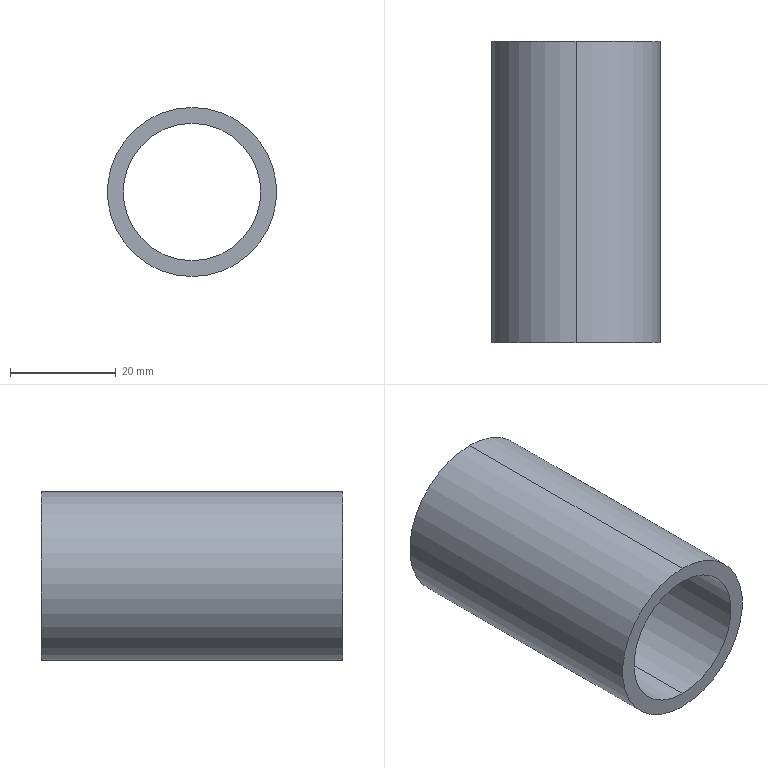Part | SolidWorks | features Chamfer 1, Extrusion 1 | 1 solid | 6 faces | box 32 x 57 x 32 mm | volume 15579 mm3 | cylinder 4 | plane 2 | commonest cylinder face diameters 26 x2 32 x2
STEP:
#1=CARTESIAN_POINT('',(0.,57.,-13.));
#2=VERTEX_POINT('',#1);
#3=CARTESIAN_POINT('',(0.,57.,13.));
#4=VERTEX_POINT('',#3);
#5=CARTESIAN_POINT('',(0.,57.,0.));
#6=DIRECTION('',(0.,1.,0.));
#7=DIRECTION('',(0.,0.,1.));
#8=AXIS2_PLACEMENT_3D('',#5,#6,#7);
#9=CIRCLE('',#8,13.);
#10=EDGE_CURVE('',#2,#4,#9,.T.);
#11=ORIENTED_EDGE('',*,*,#10,.T.);
#12=CARTESIAN_POINT('',(0.,0.,13.));
#13=VERTEX_POINT('',#12);
#14=CARTESIAN_POINT('',(0.,57.,13.));
#15=DIRECTION('',(0.,-1.,0.));
#16=VECTOR('',#15,1000.);
#17=LINE('',#14,#16);
#18=EDGE_CURVE('',#4,#13,#17,.T.);
#19=ORIENTED_EDGE('',*,*,#18,.T.);
#20=CARTESIAN_POINT('',(0.,0.,-13.));
#21=VERTEX_POINT('',#20);
#22=CARTESIAN_POINT('',(0.,0.,0.));
#23=DIRECTION('',(0.,1.,0.));
#24=DIRECTION('',(0.,0.,1.));
#25=AXIS2_PLACEMENT_3D('',#22,#23,#24);
#26=CIRCLE('',#25,13.);
#27=EDGE_CURVE('',#21,#13,#26,.T.);
#28=ORIENTED_EDGE('',*,*,#27,.F.);
#29=CARTESIAN_POINT('',(0.,57.,-13.));
#30=DIRECTION('',(0.,-1.,0.));
#31=VECTOR('',#30,1000.);
#32=LINE('',#29,#31);
#33=EDGE_CURVE('',#2,#21,#32,.T.);
#34=ORIENTED_EDGE('',*,*,#33,.F.);
#35=EDGE_LOOP('',(#11,#19,#28,#34));
#36=FACE_OUTER_BOUND('',#35,.T.);
#37=CARTESIAN_POINT('',(0.,57.,0.));
#38=DIRECTION('',(0.,-1.,0.));
#39=DIRECTION('',(0.,0.,-1.));
#40=AXIS2_PLACEMENT_3D('',#37,#38,#39);
#41=CYLINDRICAL_SURFACE('',#40,13.);
#42=ADVANCED_FACE('',(#36),#41,.F.);
#43=CARTESIAN_POINT('',(0.,57.,16.));
#44=VERTEX_POINT('',#43);
#45=CARTESIAN_POINT('',(0.,57.,-16.));
#46=VERTEX_POINT('',#45);
#47=CARTESIAN_POINT('',(0.,57.,0.));
#48=DIRECTION('',(0.,1.,0.));
#49=DIRECTION('',(0.,0.,1.));
#50=AXIS2_PLACEMENT_3D('',#47,#48,#49);
#51=CIRCLE('',#50,16.);
#52=EDGE_CURVE('',#44,#46,#51,.T.);
#53=ORIENTED_EDGE('',*,*,#52,.F.);
#54=CARTESIAN_POINT('',(0.,0.,16.));
#55=VERTEX_POINT('',#54);
#56=CARTESIAN_POINT('',(0.,57.,16.));
#57=DIRECTION('',(0.,-1.,0.));
#58=VECTOR('',#57,1000.);
#59=LINE('',#56,#58);
#60=EDGE_CURVE('',#44,#55,#59,.T.);
#61=ORIENTED_EDGE('',*,*,#60,.T.);
#62=CARTESIAN_POINT('',(0.,0.,-16.));
#63=VERTEX_POINT('',#62);
#64=CARTESIAN_POINT('',(0.,0.,0.));
#65=DIRECTION('',(0.,1.,0.));
#66=DIRECTION('',(0.,0.,1.));
#67=AXIS2_PLACEMENT_3D('',#64,#65,#66);
#68=CIRCLE('',#67,16.);
#69=EDGE_CURVE('',#55,#63,#68,.T.);
#70=ORIENTED_EDGE('',*,*,#69,.T.);
#71=CARTESIAN_POINT('',(0.,57.,-16.));
#72=DIRECTION('',(0.,-1.,0.));
#73=VECTOR('',#72,1000.);
#74=LINE('',#71,#73);
#75=EDGE_CURVE('',#46,#63,#74,.T.);
#76=ORIENTED_EDGE('',*,*,#75,.F.);
#77=EDGE_LOOP('',(#53,#61,#70,#76));
#78=FACE_OUTER_BOUND('',#77,.T.);
#79=CARTESIAN_POINT('',(0.,57.,0.));
#80=DIRECTION('',(0.,-1.,0.));
#81=DIRECTION('',(0.,0.,-1.));
#82=AXIS2_PLACEMENT_3D('',#79,#80,#81);
#83=CYLINDRICAL_SURFACE('',#82,16.);
#84=ADVANCED_FACE('',(#78),#83,.T.);
#85=CARTESIAN_POINT('',(0.,57.,0.));
#86=DIRECTION('',(0.,1.,0.));
#87=DIRECTION('',(0.,0.,1.));
#88=AXIS2_PLACEMENT_3D('',#85,#86,#87);
#89=CIRCLE('',#88,16.);
#90=EDGE_CURVE('',#46,#44,#89,.T.);
#91=ORIENTED_EDGE('',*,*,#90,.T.);
#92=ORIENTED_EDGE('',*,*,#52,.T.);
#93=EDGE_LOOP('',(#91,#92));
#94=FACE_OUTER_BOUND('',#93,.T.);
#95=ORIENTED_EDGE('',*,*,#10,.F.);
#96=CARTESIAN_POINT('',(0.,57.,0.));
#97=DIRECTION('',(0.,1.,0.));
#98=DIRECTION('',(0.,0.,1.));
#99=AXIS2_PLACEMENT_3D('',#96,#97,#98);
#100=CIRCLE('',#99,13.);
#101=EDGE_CURVE('',#4,#2,#100,.T.);
#102=ORIENTED_EDGE('',*,*,#101,.F.);
#103=EDGE_LOOP('',(#95,#102));
#104=FACE_BOUND('',#103,.T.);
#105=CARTESIAN_POINT('',(0.,57.,0.));
#106=DIRECTION('',(0.,1.,0.));
#107=DIRECTION('',(0.,0.,1.));
#108=AXIS2_PLACEMENT_3D('',#105,#106,#107);
#109=PLANE('',#108);
#110=ADVANCED_FACE('',(#94,#104),#109,.T.);
#111=CARTESIAN_POINT('',(0.,0.,0.));
#112=DIRECTION('',(0.,1.,0.));
#113=DIRECTION('',(0.,0.,1.));
#114=AXIS2_PLACEMENT_3D('',#111,#112,#113);
#115=CIRCLE('',#114,16.);
#116=EDGE_CURVE('',#63,#55,#115,.T.);
#117=ORIENTED_EDGE('',*,*,#116,.F.);
#118=ORIENTED_EDGE('',*,*,#69,.F.);
#119=EDGE_LOOP('',(#117,#118));
#120=FACE_OUTER_BOUND('',#119,.T.);
#121=ORIENTED_EDGE('',*,*,#27,.T.);
#122=CARTESIAN_POINT('',(0.,0.,0.));
#123=DIRECTION('',(0.,1.,0.));
#124=DIRECTION('',(0.,0.,1.));
#125=AXIS2_PLACEMENT_3D('',#122,#123,#124);
#126=CIRCLE('',#125,13.);
#127=EDGE_CURVE('',#13,#21,#126,.T.);
#128=ORIENTED_EDGE('',*,*,#127,.T.);
#129=EDGE_LOOP('',(#121,#128));
#130=FACE_BOUND('',#129,.T.);
#131=CARTESIAN_POINT('',(0.,0.,0.));
#132=DIRECTION('',(0.,1.,0.));
#133=DIRECTION('',(0.,0.,1.));
#134=AXIS2_PLACEMENT_3D('',#131,#132,#133);
#135=PLANE('',#134);
#136=ADVANCED_FACE('',(#120,#130),#135,.F.);
#137=ORIENTED_EDGE('',*,*,#60,.F.);
#138=ORIENTED_EDGE('',*,*,#90,.F.);
#139=ORIENTED_EDGE('',*,*,#75,.T.);
#140=ORIENTED_EDGE('',*,*,#116,.T.);
#141=EDGE_LOOP('',(#137,#138,#139,#140));
#142=FACE_OUTER_BOUND('',#141,.T.);
#143=CARTESIAN_POINT('',(0.,57.,0.));
#144=DIRECTION('',(0.,-1.,0.));
#145=DIRECTION('',(0.,0.,-1.));
#146=AXIS2_PLACEMENT_3D('',#143,#144,#145);
#147=CYLINDRICAL_SURFACE('',#146,16.);
#148=ADVANCED_FACE('',(#142),#147,.T.);
#149=ORIENTED_EDGE('',*,*,#18,.F.);
#150=ORIENTED_EDGE('',*,*,#101,.T.);
#151=ORIENTED_EDGE('',*,*,#33,.T.);
#152=ORIENTED_EDGE('',*,*,#127,.F.);
#153=EDGE_LOOP('',(#149,#150,#151,#152));
#154=FACE_OUTER_BOUND('',#153,.T.);
#155=CARTESIAN_POINT('',(0.,57.,0.));
#156=DIRECTION('',(0.,-1.,0.));
#157=DIRECTION('',(0.,0.,-1.));
#158=AXIS2_PLACEMENT_3D('',#155,#156,#157);
#159=CYLINDRICAL_SURFACE('',#158,13.);
#160=ADVANCED_FACE('',(#154),#159,.F.);
#161=CLOSED_SHELL('',(#42,#84,#110,#136,#148,#160));
#162=MANIFOLD_SOLID_BREP('',#161);
#163=CARTESIAN_POINT('',(0.,0.,0.));
#164=DIRECTION('',(0.,0.,1.));
#165=DIRECTION('',(1.,0.,0.));
#166=AXIS2_PLACEMENT_3D('',#163,#164,#165);
#167=(LENGTH_UNIT()NAMED_UNIT(*)SI_UNIT(.MILLI.,.METRE.));
#168=UNCERTAINTY_MEASURE_WITH_UNIT(LENGTH_MEASURE(0.00001),#167,'','');
#169=(NAMED_UNIT(*)PLANE_ANGLE_UNIT()SI_UNIT($,.RADIAN.));
#170=(NAMED_UNIT(*)SI_UNIT($,.STERADIAN.)SOLID_ANGLE_UNIT());
#171=(GEOMETRIC_REPRESENTATION_CONTEXT(3)GLOBAL_UNCERTAINTY_ASSIGNED_CONTEXT((#168))GLOBAL_UNIT_ASSIGNED_CONTEXT((#167,#169,#170))REPRESENTATION_CONTEXT('',''));
#172=ADVANCED_BREP_SHAPE_REPRESENTATION('',(#162,#166),#171);